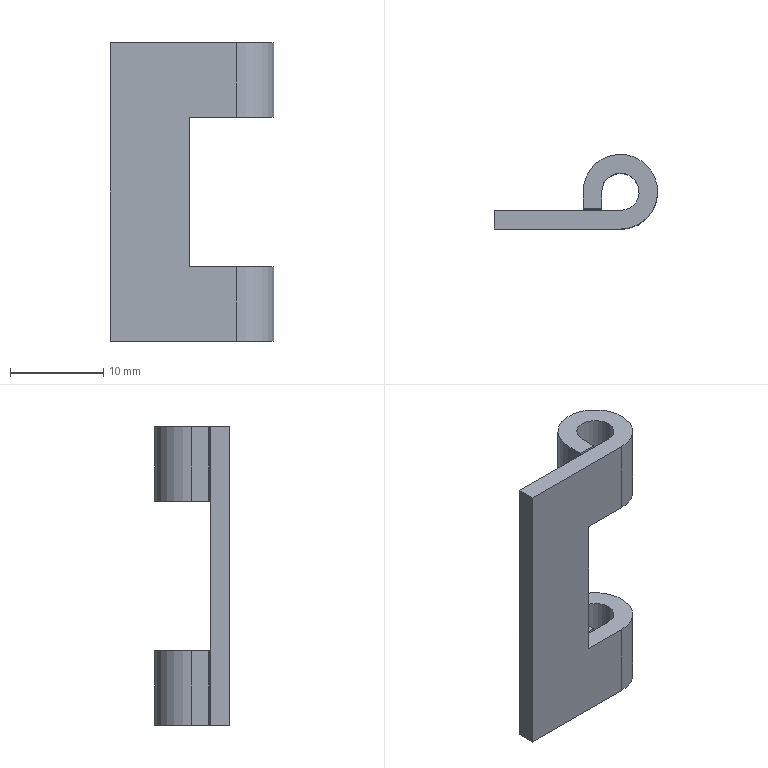Part | SolidWorks | features MirrorStock 1 | 1 solid | 18 faces | box 17.5 x 8 x 32 mm | volume 1214 mm3 | plane 14 | cylinder 4 | commonest cylinder face diameters 4 x2 8 x2
STEP:
#1=CARTESIAN_POINT('',(0.,0.,16.));
#2=VERTEX_POINT('',#1);
#3=CARTESIAN_POINT('',(-4.,4.,16.));
#4=VERTEX_POINT('',#3);
#5=CARTESIAN_POINT('',(0.,4.,16.));
#6=DIRECTION('',(0.,0.,1.));
#7=DIRECTION('',(-1.,0.,0.));
#8=AXIS2_PLACEMENT_3D('',#5,#6,#7);
#9=CIRCLE('',#8,4.);
#10=EDGE_CURVE('',#2,#4,#9,.T.);
#11=ORIENTED_EDGE('',*,*,#10,.F.);
#12=CARTESIAN_POINT('',(0.,0.,8.));
#13=VERTEX_POINT('',#12);
#14=CARTESIAN_POINT('',(0.,0.,-16.));
#15=DIRECTION('',(0.,0.,1.));
#16=VECTOR('',#15,1000.);
#17=LINE('',#14,#16);
#18=EDGE_CURVE('',#13,#2,#17,.T.);
#19=ORIENTED_EDGE('',*,*,#18,.F.);
#20=CARTESIAN_POINT('',(-4.,4.,8.));
#21=VERTEX_POINT('',#20);
#22=CARTESIAN_POINT('',(0.,4.,8.));
#23=DIRECTION('',(0.,0.,1.));
#24=DIRECTION('',(-1.,0.,0.));
#25=AXIS2_PLACEMENT_3D('',#22,#23,#24);
#26=CIRCLE('',#25,4.);
#27=EDGE_CURVE('',#13,#21,#26,.T.);
#28=ORIENTED_EDGE('',*,*,#27,.T.);
#29=CARTESIAN_POINT('',(-4.,4.,-16.));
#30=DIRECTION('',(0.,0.,-1.));
#31=VECTOR('',#30,1000.);
#32=LINE('',#29,#31);
#33=EDGE_CURVE('',#4,#21,#32,.T.);
#34=ORIENTED_EDGE('',*,*,#33,.F.);
#35=EDGE_LOOP('',(#11,#19,#28,#34));
#36=FACE_OUTER_BOUND('',#35,.T.);
#37=CARTESIAN_POINT('',(0.,4.,-16.));
#38=DIRECTION('',(0.,0.,1.));
#39=DIRECTION('',(-1.,0.,0.));
#40=AXIS2_PLACEMENT_3D('',#37,#38,#39);
#41=CYLINDRICAL_SURFACE('',#40,4.);
#42=ADVANCED_FACE('',(#36),#41,.T.);
#43=ORIENTED_EDGE('',*,*,#33,.T.);
#44=CARTESIAN_POINT('',(-4.,2.2,8.));
#45=VERTEX_POINT('',#44);
#46=CARTESIAN_POINT('',(-4.,16.,8.));
#47=DIRECTION('',(0.,-1.,0.));
#48=VECTOR('',#47,1000.);
#49=LINE('',#46,#48);
#50=EDGE_CURVE('',#21,#45,#49,.T.);
#51=ORIENTED_EDGE('',*,*,#50,.T.);
#52=CARTESIAN_POINT('',(-4.,2.2,16.));
#53=VERTEX_POINT('',#52);
#54=CARTESIAN_POINT('',(-4.,2.2,-16.));
#55=DIRECTION('',(0.,0.,-1.));
#56=VECTOR('',#55,1000.);
#57=LINE('',#54,#56);
#58=EDGE_CURVE('',#53,#45,#57,.T.);
#59=ORIENTED_EDGE('',*,*,#58,.F.);
#60=CARTESIAN_POINT('',(-4.,4.,16.));
#61=DIRECTION('',(0.,-1.,0.));
#62=VECTOR('',#61,1000.);
#63=LINE('',#60,#62);
#64=EDGE_CURVE('',#4,#53,#63,.T.);
#65=ORIENTED_EDGE('',*,*,#64,.F.);
#66=EDGE_LOOP('',(#43,#51,#59,#65));
#67=FACE_OUTER_BOUND('',#66,.T.);
#68=CARTESIAN_POINT('',(-4.,4.,-16.));
#69=DIRECTION('',(1.,0.,0.));
#70=DIRECTION('',(0.,0.,1.));
#71=AXIS2_PLACEMENT_3D('',#68,#69,#70);
#72=PLANE('',#71);
#73=ADVANCED_FACE('',(#67),#72,.F.);
#74=ORIENTED_EDGE('',*,*,#58,.T.);
#75=CARTESIAN_POINT('',(-2.,2.2,8.));
#76=VERTEX_POINT('',#75);
#77=CARTESIAN_POINT('',(6.,2.2,8.));
#78=DIRECTION('',(1.,0.,0.));
#79=VECTOR('',#78,1000.);
#80=LINE('',#77,#79);
#81=EDGE_CURVE('',#45,#76,#80,.T.);
#82=ORIENTED_EDGE('',*,*,#81,.T.);
#83=CARTESIAN_POINT('',(-2.,2.2,16.));
#84=VERTEX_POINT('',#83);
#85=CARTESIAN_POINT('',(-2.,2.2,-16.));
#86=DIRECTION('',(0.,0.,-1.));
#87=VECTOR('',#86,1000.);
#88=LINE('',#85,#87);
#89=EDGE_CURVE('',#84,#76,#88,.T.);
#90=ORIENTED_EDGE('',*,*,#89,.F.);
#91=CARTESIAN_POINT('',(0.,2.2,16.));
#92=DIRECTION('',(1.,0.,0.));
#93=VECTOR('',#92,1000.);
#94=LINE('',#91,#93);
#95=EDGE_CURVE('',#53,#84,#94,.T.);
#96=ORIENTED_EDGE('',*,*,#95,.F.);
#97=EDGE_LOOP('',(#74,#82,#90,#96));
#98=FACE_OUTER_BOUND('',#97,.T.);
#99=CARTESIAN_POINT('',(-4.,2.2,-16.));
#100=DIRECTION('',(0.,1.,0.));
#101=DIRECTION('',(0.,0.,-1.));
#102=AXIS2_PLACEMENT_3D('',#99,#100,#101);
#103=PLANE('',#102);
#104=ADVANCED_FACE('',(#98),#103,.F.);
#105=ORIENTED_EDGE('',*,*,#89,.T.);
#106=CARTESIAN_POINT('',(-2.,4.,8.));
#107=VERTEX_POINT('',#106);
#108=CARTESIAN_POINT('',(-2.,16.,8.));
#109=DIRECTION('',(0.,1.,0.));
#110=VECTOR('',#109,1000.);
#111=LINE('',#108,#110);
#112=EDGE_CURVE('',#76,#107,#111,.T.);
#113=ORIENTED_EDGE('',*,*,#112,.T.);
#114=CARTESIAN_POINT('',(-2.,4.,16.));
#115=VERTEX_POINT('',#114);
#116=CARTESIAN_POINT('',(-2.,4.,-16.));
#117=DIRECTION('',(0.,0.,-1.));
#118=VECTOR('',#117,1000.);
#119=LINE('',#116,#118);
#120=EDGE_CURVE('',#115,#107,#119,.T.);
#121=ORIENTED_EDGE('',*,*,#120,.F.);
#122=CARTESIAN_POINT('',(-2.,4.,16.));
#123=DIRECTION('',(0.,1.,0.));
#124=VECTOR('',#123,1000.);
#125=LINE('',#122,#124);
#126=EDGE_CURVE('',#84,#115,#125,.T.);
#127=ORIENTED_EDGE('',*,*,#126,.F.);
#128=EDGE_LOOP('',(#105,#113,#121,#127));
#129=FACE_OUTER_BOUND('',#128,.T.);
#130=CARTESIAN_POINT('',(-2.,2.2,-16.));
#131=DIRECTION('',(-1.,0.,0.));
#132=DIRECTION('',(0.,0.,-1.));
#133=AXIS2_PLACEMENT_3D('',#130,#131,#132);
#134=PLANE('',#133);
#135=ADVANCED_FACE('',(#129),#134,.F.);
#136=CARTESIAN_POINT('',(-2.,4.,-8.));
#137=VERTEX_POINT('',#136);
#138=CARTESIAN_POINT('',(-2.,4.,-16.));
#139=VERTEX_POINT('',#138);
#140=CARTESIAN_POINT('',(-2.,4.,-16.));
#141=DIRECTION('',(0.,0.,-1.));
#142=VECTOR('',#141,1000.);
#143=LINE('',#140,#142);
#144=EDGE_CURVE('',#137,#139,#143,.T.);
#145=ORIENTED_EDGE('',*,*,#144,.F.);
#146=CARTESIAN_POINT('',(-2.,2.2,-8.));
#147=VERTEX_POINT('',#146);
#148=CARTESIAN_POINT('',(-2.,16.,-8.));
#149=DIRECTION('',(0.,-1.,0.));
#150=VECTOR('',#149,1000.);
#151=LINE('',#148,#150);
#152=EDGE_CURVE('',#137,#147,#151,.T.);
#153=ORIENTED_EDGE('',*,*,#152,.T.);
#154=CARTESIAN_POINT('',(-2.,2.2,-16.));
#155=VERTEX_POINT('',#154);
#156=CARTESIAN_POINT('',(-2.,2.2,-16.));
#157=DIRECTION('',(0.,0.,1.));
#158=VECTOR('',#157,1000.);
#159=LINE('',#156,#158);
#160=EDGE_CURVE('',#155,#147,#159,.T.);
#161=ORIENTED_EDGE('',*,*,#160,.F.);
#162=CARTESIAN_POINT('',(-2.,4.,-16.));
#163=DIRECTION('',(0.,1.,0.));
#164=VECTOR('',#163,1000.);
#165=LINE('',#162,#164);
#166=EDGE_CURVE('',#155,#139,#165,.T.);
#167=ORIENTED_EDGE('',*,*,#166,.T.);
#168=EDGE_LOOP('',(#145,#153,#161,#167));
#169=FACE_OUTER_BOUND('',#168,.T.);
#170=CARTESIAN_POINT('',(-2.,2.2,-16.));
#171=DIRECTION('',(-1.,0.,0.));
#172=DIRECTION('',(0.,0.,-1.));
#173=AXIS2_PLACEMENT_3D('',#170,#171,#172);
#174=PLANE('',#173);
#175=ADVANCED_FACE('',(#169),#174,.F.);
#176=ORIENTED_EDGE('',*,*,#160,.T.);
#177=CARTESIAN_POINT('',(-4.,2.2,-8.));
#178=VERTEX_POINT('',#177);
#179=CARTESIAN_POINT('',(-5.,2.2,-8.));
#180=DIRECTION('',(-1.,0.,0.));
#181=VECTOR('',#180,1000.);
#182=LINE('',#179,#181);
#183=EDGE_CURVE('',#147,#178,#182,.T.);
#184=ORIENTED_EDGE('',*,*,#183,.T.);
#185=CARTESIAN_POINT('',(-4.,2.2,-16.));
#186=VERTEX_POINT('',#185);
#187=CARTESIAN_POINT('',(-4.,2.2,-16.));
#188=DIRECTION('',(0.,0.,1.));
#189=VECTOR('',#188,1000.);
#190=LINE('',#187,#189);
#191=EDGE_CURVE('',#186,#178,#190,.T.);
#192=ORIENTED_EDGE('',*,*,#191,.F.);
#193=CARTESIAN_POINT('',(0.,2.2,-16.));
#194=DIRECTION('',(1.,0.,0.));
#195=VECTOR('',#194,1000.);
#196=LINE('',#193,#195);
#197=EDGE_CURVE('',#186,#155,#196,.T.);
#198=ORIENTED_EDGE('',*,*,#197,.T.);
#199=EDGE_LOOP('',(#176,#184,#192,#198));
#200=FACE_OUTER_BOUND('',#199,.T.);
#201=CARTESIAN_POINT('',(-4.,2.2,-16.));
#202=DIRECTION('',(0.,1.,0.));
#203=DIRECTION('',(0.,0.,-1.));
#204=AXIS2_PLACEMENT_3D('',#201,#202,#203);
#205=PLANE('',#204);
#206=ADVANCED_FACE('',(#200),#205,.F.);
#207=ORIENTED_EDGE('',*,*,#191,.T.);
#208=CARTESIAN_POINT('',(-4.,4.,-8.));
#209=VERTEX_POINT('',#208);
#210=CARTESIAN_POINT('',(-4.,16.,-8.));
#211=DIRECTION('',(0.,1.,0.));
#212=VECTOR('',#211,1000.);
#213=LINE('',#210,#212);
#214=EDGE_CURVE('',#178,#209,#213,.T.);
#215=ORIENTED_EDGE('',*,*,#214,.T.);
#216=CARTESIAN_POINT('',(-4.,4.,-16.));
#217=VERTEX_POINT('',#216);
#218=CARTESIAN_POINT('',(-4.,4.,-16.));
#219=DIRECTION('',(0.,0.,-1.));
#220=VECTOR('',#219,1000.);
#221=LINE('',#218,#220);
#222=EDGE_CURVE('',#209,#217,#221,.T.);
#223=ORIENTED_EDGE('',*,*,#222,.T.);
#224=CARTESIAN_POINT('',(-4.,4.,-16.));
#225=DIRECTION('',(0.,-1.,0.));
#226=VECTOR('',#225,1000.);
#227=LINE('',#224,#226);
#228=EDGE_CURVE('',#217,#186,#227,.T.);
#229=ORIENTED_EDGE('',*,*,#228,.T.);
#230=EDGE_LOOP('',(#207,#215,#223,#229));
#231=FACE_OUTER_BOUND('',#230,.T.);
#232=CARTESIAN_POINT('',(-4.,4.,-16.));
#233=DIRECTION('',(1.,0.,0.));
#234=DIRECTION('',(0.,0.,1.));
#235=AXIS2_PLACEMENT_3D('',#232,#233,#234);
#236=PLANE('',#235);
#237=ADVANCED_FACE('',(#231),#236,.F.);
#238=CARTESIAN_POINT('',(0.,0.,-16.));
#239=VERTEX_POINT('',#238);
#240=CARTESIAN_POINT('',(0.,4.,-16.));
#241=DIRECTION('',(0.,0.,1.));
#242=DIRECTION('',(-1.,0.,0.));
#243=AXIS2_PLACEMENT_3D('',#240,#241,#242);
#244=CIRCLE('',#243,4.);
#245=EDGE_CURVE('',#239,#217,#244,.T.);
#246=ORIENTED_EDGE('',*,*,#245,.T.);
#247=ORIENTED_EDGE('',*,*,#222,.F.);
#248=CARTESIAN_POINT('',(0.,0.,-8.));
#249=VERTEX_POINT('',#248);
#250=CARTESIAN_POINT('',(0.,4.,-8.));
#251=DIRECTION('',(0.,0.,-1.));
#252=DIRECTION('',(-1.,0.,0.));
#253=AXIS2_PLACEMENT_3D('',#250,#251,#252);
#254=CIRCLE('',#253,4.);
#255=EDGE_CURVE('',#209,#249,#254,.T.);
#256=ORIENTED_EDGE('',*,*,#255,.T.);
#257=CARTESIAN_POINT('',(0.,0.,-16.));
#258=DIRECTION('',(0.,0.,1.));
#259=VECTOR('',#258,1000.);
#260=LINE('',#257,#259);
#261=EDGE_CURVE('',#239,#249,#260,.T.);
#262=ORIENTED_EDGE('',*,*,#261,.F.);
#263=EDGE_LOOP('',(#246,#247,#256,#262));
#264=FACE_OUTER_BOUND('',#263,.T.);
#265=CARTESIAN_POINT('',(0.,4.,-16.));
#266=DIRECTION('',(0.,0.,1.));
#267=DIRECTION('',(-1.,0.,0.));
#268=AXIS2_PLACEMENT_3D('',#265,#266,#267);
#269=CYLINDRICAL_SURFACE('',#268,4.);
#270=ADVANCED_FACE('',(#264),#269,.T.);
#271=ORIENTED_EDGE('',*,*,#261,.T.);
#272=CARTESIAN_POINT('',(-5.,0.,-8.));
#273=VERTEX_POINT('',#272);
#274=CARTESIAN_POINT('',(-5.,0.,-8.));
#275=DIRECTION('',(-1.,0.,0.));
#276=VECTOR('',#275,1000.);
#277=LINE('',#274,#276);
#278=EDGE_CURVE('',#249,#273,#277,.T.);
#279=ORIENTED_EDGE('',*,*,#278,.T.);
#280=CARTESIAN_POINT('',(-5.,0.,8.));
#281=VERTEX_POINT('',#280);
#282=CARTESIAN_POINT('',(-5.,0.,8.));
#283=DIRECTION('',(0.,0.,1.));
#284=VECTOR('',#283,1000.);
#285=LINE('',#282,#284);
#286=EDGE_CURVE('',#273,#281,#285,.T.);
#287=ORIENTED_EDGE('',*,*,#286,.T.);
#288=CARTESIAN_POINT('',(6.,0.,8.));
#289=DIRECTION('',(1.,0.,0.));
#290=VECTOR('',#289,1000.);
#291=LINE('',#288,#290);
#292=EDGE_CURVE('',#281,#13,#291,.T.);
#293=ORIENTED_EDGE('',*,*,#292,.T.);
#294=ORIENTED_EDGE('',*,*,#18,.T.);
#295=CARTESIAN_POINT('',(-13.5,0.,16.));
#296=VERTEX_POINT('',#295);
#297=CARTESIAN_POINT('',(0.,0.,16.));
#298=DIRECTION('',(1.,0.,0.));
#299=VECTOR('',#298,1000.);
#300=LINE('',#297,#299);
#301=EDGE_CURVE('',#296,#2,#300,.T.);
#302=ORIENTED_EDGE('',*,*,#301,.F.);
#303=CARTESIAN_POINT('',(-13.5,0.,-16.));
#304=VERTEX_POINT('',#303);
#305=CARTESIAN_POINT('',(-13.5,0.,-16.));
#306=DIRECTION('',(0.,0.,1.));
#307=VECTOR('',#306,1000.);
#308=LINE('',#305,#307);
#309=EDGE_CURVE('',#304,#296,#308,.T.);
#310=ORIENTED_EDGE('',*,*,#309,.F.);
#311=CARTESIAN_POINT('',(0.,0.,-16.));
#312=DIRECTION('',(1.,0.,0.));
#313=VECTOR('',#312,1000.);
#314=LINE('',#311,#313);
#315=EDGE_CURVE('',#304,#239,#314,.T.);
#316=ORIENTED_EDGE('',*,*,#315,.T.);
#317=EDGE_LOOP('',(#271,#279,#287,#293,#294,#302,#310,#316));
#318=FACE_OUTER_BOUND('',#317,.T.);
#319=CARTESIAN_POINT('',(-13.5,0.,-16.));
#320=DIRECTION('',(0.,1.,0.));
#321=DIRECTION('',(0.,0.,-1.));
#322=AXIS2_PLACEMENT_3D('',#319,#320,#321);
#323=PLANE('',#322);
#324=ADVANCED_FACE('',(#318),#323,.F.);
#325=CARTESIAN_POINT('',(0.,2.,-8.));
#326=VERTEX_POINT('',#325);
#327=CARTESIAN_POINT('',(0.,4.,-8.));
#328=DIRECTION('',(0.,0.,1.));
#329=DIRECTION('',(-1.,0.,0.));
#330=AXIS2_PLACEMENT_3D('',#327,#328,#329);
#331=CIRCLE('',#330,2.);
#332=EDGE_CURVE('',#326,#137,#331,.T.);
#333=ORIENTED_EDGE('',*,*,#332,.T.);
#334=ORIENTED_EDGE('',*,*,#144,.T.);
#335=CARTESIAN_POINT('',(0.,2.,-16.));
#336=VERTEX_POINT('',#335);
#337=CARTESIAN_POINT('',(0.,4.,-16.));
#338=DIRECTION('',(0.,0.,-1.));
#339=DIRECTION('',(-1.,0.,0.));
#340=AXIS2_PLACEMENT_3D('',#337,#338,#339);
#341=CIRCLE('',#340,2.);
#342=EDGE_CURVE('',#139,#336,#341,.T.);
#343=ORIENTED_EDGE('',*,*,#342,.T.);
#344=CARTESIAN_POINT('',(0.,2.,-16.));
#345=DIRECTION('',(0.,0.,-1.));
#346=VECTOR('',#345,1000.);
#347=LINE('',#344,#346);
#348=EDGE_CURVE('',#326,#336,#347,.T.);
#349=ORIENTED_EDGE('',*,*,#348,.F.);
#350=EDGE_LOOP('',(#333,#334,#343,#349));
#351=FACE_OUTER_BOUND('',#350,.T.);
#352=CARTESIAN_POINT('',(0.,4.,-16.));
#353=DIRECTION('',(0.,0.,1.));
#354=DIRECTION('',(-1.,0.,0.));
#355=AXIS2_PLACEMENT_3D('',#352,#353,#354);
#356=CYLINDRICAL_SURFACE('',#355,2.);
#357=ADVANCED_FACE('',(#351),#356,.F.);
#358=ORIENTED_EDGE('',*,*,#166,.F.);
#359=ORIENTED_EDGE('',*,*,#197,.F.);
#360=ORIENTED_EDGE('',*,*,#228,.F.);
#361=ORIENTED_EDGE('',*,*,#245,.F.);
#362=ORIENTED_EDGE('',*,*,#315,.F.);
#363=CARTESIAN_POINT('',(-13.5,2.,-16.));
#364=VERTEX_POINT('',#363);
#365=CARTESIAN_POINT('',(-13.5,2.,-16.));
#366=DIRECTION('',(0.,-1.,0.));
#367=VECTOR('',#366,1000.);
#368=LINE('',#365,#367);
#369=EDGE_CURVE('',#364,#304,#368,.T.);
#370=ORIENTED_EDGE('',*,*,#369,.F.);
#371=CARTESIAN_POINT('',(0.,2.,-16.));
#372=DIRECTION('',(-1.,0.,0.));
#373=VECTOR('',#372,1000.);
#374=LINE('',#371,#373);
#375=EDGE_CURVE('',#336,#364,#374,.T.);
#376=ORIENTED_EDGE('',*,*,#375,.F.);
#377=ORIENTED_EDGE('',*,*,#342,.F.);
#378=EDGE_LOOP('',(#358,#359,#360,#361,#362,#370,#376,#377));
#379=FACE_OUTER_BOUND('',#378,.T.);
#380=CARTESIAN_POINT('',(0.,4.,-16.));
#381=DIRECTION('',(0.,0.,-1.));
#382=DIRECTION('',(1.,0.,0.));
#383=AXIS2_PLACEMENT_3D('',#380,#381,#382);
#384=PLANE('',#383);
#385=ADVANCED_FACE('',(#379),#384,.T.);
#386=ORIENTED_EDGE('',*,*,#309,.T.);
#387=CARTESIAN_POINT('',(-13.5,2.,16.));
#388=VERTEX_POINT('',#387);
#389=CARTESIAN_POINT('',(-13.5,4.,16.));
#390=DIRECTION('',(0.,-1.,0.));
#391=VECTOR('',#390,1000.);
#392=LINE('',#389,#391);
#393=EDGE_CURVE('',#388,#296,#392,.T.);
#394=ORIENTED_EDGE('',*,*,#393,.F.);
#395=CARTESIAN_POINT('',(-13.5,2.,-16.));
#396=DIRECTION('',(0.,0.,1.));
#397=VECTOR('',#396,1000.);
#398=LINE('',#395,#397);
#399=EDGE_CURVE('',#364,#388,#398,.T.);
#400=ORIENTED_EDGE('',*,*,#399,.F.);
#401=ORIENTED_EDGE('',*,*,#369,.T.);
#402=EDGE_LOOP('',(#386,#394,#400,#401));
#403=FACE_OUTER_BOUND('',#402,.T.);
#404=CARTESIAN_POINT('',(-13.5,2.,-16.));
#405=DIRECTION('',(1.,0.,0.));
#406=DIRECTION('',(0.,0.,1.));
#407=AXIS2_PLACEMENT_3D('',#404,#405,#406);
#408=PLANE('',#407);
#409=ADVANCED_FACE('',(#403),#408,.F.);
#410=CARTESIAN_POINT('',(0.,2.,16.));
#411=VERTEX_POINT('',#410);
#412=CARTESIAN_POINT('',(0.,4.,16.));
#413=DIRECTION('',(0.,0.,1.));
#414=DIRECTION('',(-1.,0.,0.));
#415=AXIS2_PLACEMENT_3D('',#412,#413,#414);
#416=CIRCLE('',#415,2.);
#417=EDGE_CURVE('',#411,#115,#416,.T.);
#418=ORIENTED_EDGE('',*,*,#417,.F.);
#419=CARTESIAN_POINT('',(0.,2.,16.));
#420=DIRECTION('',(1.,0.,0.));
#421=VECTOR('',#420,1000.);
#422=LINE('',#419,#421);
#423=EDGE_CURVE('',#388,#411,#422,.T.);
#424=ORIENTED_EDGE('',*,*,#423,.F.);
#425=ORIENTED_EDGE('',*,*,#393,.T.);
#426=ORIENTED_EDGE('',*,*,#301,.T.);
#427=ORIENTED_EDGE('',*,*,#10,.T.);
#428=ORIENTED_EDGE('',*,*,#64,.T.);
#429=ORIENTED_EDGE('',*,*,#95,.T.);
#430=ORIENTED_EDGE('',*,*,#126,.T.);
#431=EDGE_LOOP('',(#418,#424,#425,#426,#427,#428,#429,#430));
#432=FACE_OUTER_BOUND('',#431,.T.);
#433=CARTESIAN_POINT('',(0.,4.,16.));
#434=DIRECTION('',(0.,0.,-1.));
#435=DIRECTION('',(1.,0.,0.));
#436=AXIS2_PLACEMENT_3D('',#433,#434,#435);
#437=PLANE('',#436);
#438=ADVANCED_FACE('',(#432),#437,.F.);
#439=CARTESIAN_POINT('',(0.,2.,8.));
#440=VERTEX_POINT('',#439);
#441=CARTESIAN_POINT('',(0.,4.,8.));
#442=DIRECTION('',(0.,0.,-1.));
#443=DIRECTION('',(-1.,0.,0.));
#444=AXIS2_PLACEMENT_3D('',#441,#442,#443);
#445=CIRCLE('',#444,2.);
#446=EDGE_CURVE('',#107,#440,#445,.T.);
#447=ORIENTED_EDGE('',*,*,#446,.T.);
#448=CARTESIAN_POINT('',(0.,2.,-16.));
#449=DIRECTION('',(0.,0.,-1.));
#450=VECTOR('',#449,1000.);
#451=LINE('',#448,#450);
#452=EDGE_CURVE('',#411,#440,#451,.T.);
#453=ORIENTED_EDGE('',*,*,#452,.F.);
#454=ORIENTED_EDGE('',*,*,#417,.T.);
#455=ORIENTED_EDGE('',*,*,#120,.T.);
#456=EDGE_LOOP('',(#447,#453,#454,#455));
#457=FACE_OUTER_BOUND('',#456,.T.);
#458=CARTESIAN_POINT('',(0.,4.,-16.));
#459=DIRECTION('',(0.,0.,1.));
#460=DIRECTION('',(-1.,0.,0.));
#461=AXIS2_PLACEMENT_3D('',#458,#459,#460);
#462=CYLINDRICAL_SURFACE('',#461,2.);
#463=ADVANCED_FACE('',(#457),#462,.F.);
#464=ORIENTED_EDGE('',*,*,#112,.F.);
#465=ORIENTED_EDGE('',*,*,#81,.F.);
#466=ORIENTED_EDGE('',*,*,#50,.F.);
#467=ORIENTED_EDGE('',*,*,#27,.F.);
#468=ORIENTED_EDGE('',*,*,#292,.F.);
#469=CARTESIAN_POINT('',(-5.,2.,8.));
#470=VERTEX_POINT('',#469);
#471=CARTESIAN_POINT('',(-5.,16.,8.));
#472=DIRECTION('',(0.,1.,0.));
#473=VECTOR('',#472,1000.);
#474=LINE('',#471,#473);
#475=EDGE_CURVE('',#281,#470,#474,.T.);
#476=ORIENTED_EDGE('',*,*,#475,.T.);
#477=CARTESIAN_POINT('',(0.,2.,8.));
#478=DIRECTION('',(-1.,0.,0.));
#479=VECTOR('',#478,1000.);
#480=LINE('',#477,#479);
#481=EDGE_CURVE('',#440,#470,#480,.T.);
#482=ORIENTED_EDGE('',*,*,#481,.F.);
#483=ORIENTED_EDGE('',*,*,#446,.F.);
#484=EDGE_LOOP('',(#464,#465,#466,#467,#468,#476,#482,#483));
#485=FACE_OUTER_BOUND('',#484,.T.);
#486=CARTESIAN_POINT('',(6.,16.,8.));
#487=DIRECTION('',(0.,0.,-1.));
#488=DIRECTION('',(1.,0.,0.));
#489=AXIS2_PLACEMENT_3D('',#486,#487,#488);
#490=PLANE('',#489);
#491=ADVANCED_FACE('',(#485),#490,.T.);
#492=ORIENTED_EDGE('',*,*,#286,.F.);
#493=CARTESIAN_POINT('',(-5.,2.,-8.));
#494=VERTEX_POINT('',#493);
#495=CARTESIAN_POINT('',(-5.,16.,-8.));
#496=DIRECTION('',(0.,1.,0.));
#497=VECTOR('',#496,1000.);
#498=LINE('',#495,#497);
#499=EDGE_CURVE('',#273,#494,#498,.T.);
#500=ORIENTED_EDGE('',*,*,#499,.T.);
#501=CARTESIAN_POINT('',(-5.,2.,-16.));
#502=DIRECTION('',(0.,0.,-1.));
#503=VECTOR('',#502,1000.);
#504=LINE('',#501,#503);
#505=EDGE_CURVE('',#470,#494,#504,.T.);
#506=ORIENTED_EDGE('',*,*,#505,.F.);
#507=ORIENTED_EDGE('',*,*,#475,.F.);
#508=EDGE_LOOP('',(#492,#500,#506,#507));
#509=FACE_OUTER_BOUND('',#508,.T.);
#510=CARTESIAN_POINT('',(-5.,16.,8.));
#511=DIRECTION('',(1.,0.,0.));
#512=DIRECTION('',(0.,0.,1.));
#513=AXIS2_PLACEMENT_3D('',#510,#511,#512);
#514=PLANE('',#513);
#515=ADVANCED_FACE('',(#509),#514,.T.);
#516=ORIENTED_EDGE('',*,*,#278,.F.);
#517=ORIENTED_EDGE('',*,*,#255,.F.);
#518=ORIENTED_EDGE('',*,*,#214,.F.);
#519=ORIENTED_EDGE('',*,*,#183,.F.);
#520=ORIENTED_EDGE('',*,*,#152,.F.);
#521=ORIENTED_EDGE('',*,*,#332,.F.);
#522=CARTESIAN_POINT('',(0.,2.,-8.));
#523=DIRECTION('',(1.,0.,0.));
#524=VECTOR('',#523,1000.);
#525=LINE('',#522,#524);
#526=EDGE_CURVE('',#494,#326,#525,.T.);
#527=ORIENTED_EDGE('',*,*,#526,.F.);
#528=ORIENTED_EDGE('',*,*,#499,.F.);
#529=EDGE_LOOP('',(#516,#517,#518,#519,#520,#521,#527,#528));
#530=FACE_OUTER_BOUND('',#529,.T.);
#531=CARTESIAN_POINT('',(-5.,16.,-8.));
#532=DIRECTION('',(0.,0.,1.));
#533=DIRECTION('',(-1.,0.,0.));
#534=AXIS2_PLACEMENT_3D('',#531,#532,#533);
#535=PLANE('',#534);
#536=ADVANCED_FACE('',(#530),#535,.T.);
#537=ORIENTED_EDGE('',*,*,#505,.T.);
#538=ORIENTED_EDGE('',*,*,#526,.T.);
#539=ORIENTED_EDGE('',*,*,#348,.T.);
#540=ORIENTED_EDGE('',*,*,#375,.T.);
#541=ORIENTED_EDGE('',*,*,#399,.T.);
#542=ORIENTED_EDGE('',*,*,#423,.T.);
#543=ORIENTED_EDGE('',*,*,#452,.T.);
#544=ORIENTED_EDGE('',*,*,#481,.T.);
#545=EDGE_LOOP('',(#537,#538,#539,#540,#541,#542,#543,#544));
#546=FACE_OUTER_BOUND('',#545,.T.);
#547=CARTESIAN_POINT('',(0.,2.,-16.));
#548=DIRECTION('',(0.,-1.,0.));
#549=DIRECTION('',(0.,0.,1.));
#550=AXIS2_PLACEMENT_3D('',#547,#548,#549);
#551=PLANE('',#550);
#552=ADVANCED_FACE('',(#546),#551,.F.);
#553=CLOSED_SHELL('',(#42,#73,#104,#135,#175,#206,#237,#270,#324,#357,#385,#409,#438,#463,#491,#515,#536,#552));
#554=MANIFOLD_SOLID_BREP('',#553);
#555=CARTESIAN_POINT('',(0.,0.,0.));
#556=DIRECTION('',(0.,0.,1.));
#557=DIRECTION('',(1.,0.,0.));
#558=AXIS2_PLACEMENT_3D('',#555,#556,#557);
#559=(LENGTH_UNIT()NAMED_UNIT(*)SI_UNIT(.MILLI.,.METRE.));
#560=UNCERTAINTY_MEASURE_WITH_UNIT(LENGTH_MEASURE(0.00001),#559,'','');
#561=(NAMED_UNIT(*)PLANE_ANGLE_UNIT()SI_UNIT($,.RADIAN.));
#562=(NAMED_UNIT(*)SI_UNIT($,.STERADIAN.)SOLID_ANGLE_UNIT());
#563=(GEOMETRIC_REPRESENTATION_CONTEXT(3)GLOBAL_UNCERTAINTY_ASSIGNED_CONTEXT((#560))GLOBAL_UNIT_ASSIGNED_CONTEXT((#559,#561,#562))REPRESENTATION_CONTEXT('',''));
#564=ADVANCED_BREP_SHAPE_REPRESENTATION('',(#554,#558),#563);